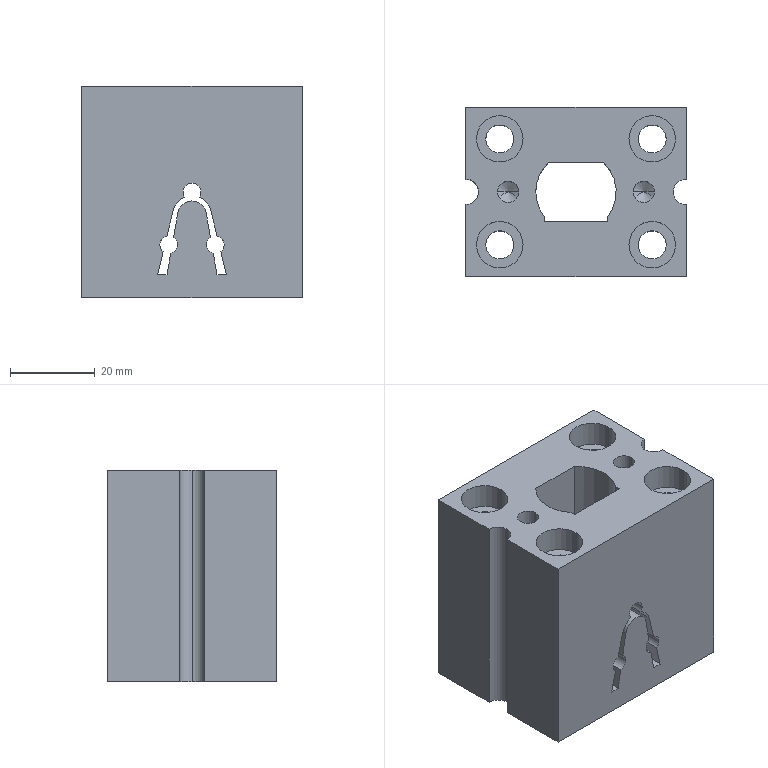Part | STEP file | secondary slingshot input seat | 1 solid | 90 faces | box 52 x 40 x 50 mm | volume 79247 mm3 | plane 44 | cylinder 42 | cone 4 | commonest cylinder face diameters 4.2 x10 6.6 x8 11 x8 5 x4 9.2 x4 6 x3